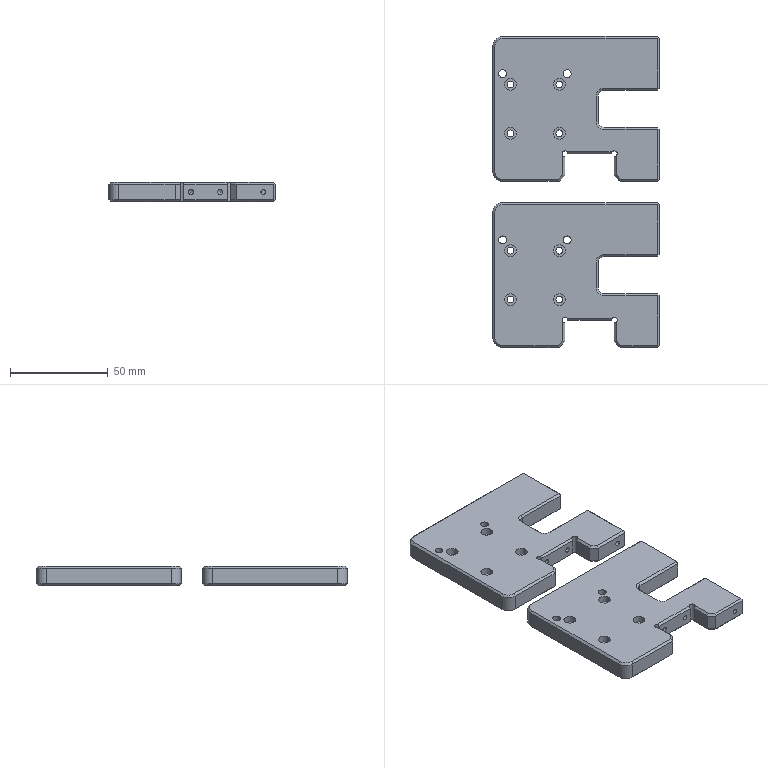NC program | NX | posted with a generic post | part box 85 x 159 x 10 mm
Whole program:
N10 G17 G21 G94 G90
(HOLE_MILLING_COPY_COPY_1 , TOOL : D4)
N12 T15 M6
N14 G54
N16 G17 G0 G90 X-30. Y0. B0. C0. S7500 M3
N18 G43 Z30. H15
N20 Z0.5
N22 G94 G3 X-30.45 Y0.45 R0.45 F1200.
N24 X-30.9 Y0. R0.45
N26 X-30.9 Y0. Z0.2 I0.9 J0.
N28 X-30.9 Y0. Z-0.1 I0.9 J0.
N30 X-30.9 Y0. Z-0.4 I0.9 J0.
N32 X-30.9 Y0. Z-0.7 I0.9 J0.
N34 X-30.9 Y0. Z-1. I0.9 J0.
N36 X-30.9 Y0. Z-1.3 I0.9 J0.
N38 X-30.9 Y0. Z-1.6 I0.9 J0.
N40 X-30.9 Y0. Z-1.9 I0.9 J0.
N42 X-30.9 Y0. Z-2.2 I0.9 J0.
N44 X-30.9 Y0. Z-2.5 I0.9 J0.
N46 X-30.9 Y0. Z-2.8 I0.9 J0.
N48 X-30.9 Y0. Z-3.1 I0.9 J0.
N50 X-30.9 Y0. Z-3.4 I0.9 J0.
N52 X-30.9 Y0. Z-3.7 I0.9 J0.
N54 X-30.9 Y0. Z-4. I0.9 J0.
N56 X-30.9 Y0. Z-4.3 I0.9 J0.
N58 X-30.9 Y0. Z-4.6 I0.9 J0.
N60 X-30.9 Y0. Z-4.9 I0.9 J0.
N62 X-30.9 Y0. Z-5.2 I0.9 J0.
N64 X-30.9 Y0. Z-5.5 I0.9 J0.
N66 X-30.9 Y0. Z-5.8 I0.9 J0.
N68 X-30.9 Y0. Z-6.1 I0.9 J0.
N70 X-30.9 Y0. Z-6.4 I0.9 J0.
N72 X-30.9 Y0. Z-6.7 I0.9 J0.
N74 X-30.9 Y0. Z-7. I0.9 J0.
N76 X-30.9 Y0. Z-7.3 I0.9 J0.
N78 X-30.9 Y0. Z-7.6 I0.9 J0.
N80 X-30.9 Y0. Z-7.9 I0.9 J0.
N82 X-30.9 Y0. Z-8.2 I0.9 J0.
N84 X-30.9 Y0. Z-8.5 I0.9 J0.
N86 X-30.9 Y0. Z-8.8 I0.9 J0.
N88 X-30.9 Y0. Z-9.1 I0.9 J0.
N90 X-30.9 Y0. Z-9.4 I0.9 J0.
N92 X-30.9 Y0. Z-9.7 I0.9 J0.
N94 X-30.9 Y0. Z-10. I0.9 J0.
N96 X-30.9 Y0. Z-10.3 I0.9 J0.
N98 X-30.9 Y0. Z-10.6 I0.9 J0.
N100 X-30.9 Y0. Z-10.9 I0.9 J0.
N102 X-30.9 Y0. Z-11.2 I0.9 J0.
N104 X-30.9 Y0. Z-11.5 I0.9 J0.
N106 X-30.9 Y0. Z-11.8 I0.9 J0.
N108 X-30.9 Y0. Z-12.1 I0.9 J0.
N110 X-30.9 Y0. Z-12.4 I0.9 J0.
N112 X-30.9 Y0. Z-12.7 I0.9 J0.
N114 X-30.9 Y0. Z-13. I0.9 J0.
N116 X-30.9 Y0. Z-13.3 I0.9 J0.
N118 X-30.9 Y0. Z-13.6 I0.9 J0.
N120 X-30.9 Y0. Z-13.9 I0.9 J0.
N122 X-30.9 Y0. Z-14.2 I0.9 J0.
N124 X-30.9 Y0. Z-14.5 I0.9 J0.
N126 X-30.9 Y0. Z-14.8 I0.9 J0.
N128 X-30.9 Y0. Z-15.1 I0.9 J0.
N130 X-30.9 Y0. Z-15.4 I0.9 J0.
N132 X-30.9 Y0. Z-15.7 I0.9 J0.
N134 X-30.9 Y0. Z-16. I0.9 J0.
N136 X-30. Y-0.9 R0.9
N138 X-30.9 Y0. R-0.9
N140 X-30.45 Y-0.45 R0.45
N142 X-30. Y0. R0.45
N144 G0 Z30.
N146 X30.
N148 Z0.5
N150 G3 X29.55 Y0.45 R0.45
N152 X29.1 Y0. R0.45
N154 X29.1 Y0. Z0.2 I0.9 J0.
N156 X29.1 Y0. Z-0.1 I0.9 J0.
N158 X29.1 Y0. Z-0.4 I0.9 J0.
N160 X29.1 Y0. Z-0.7 I0.9 J0.
N162 X29.1 Y0. Z-1. I0.9 J0.
N164 X29.1 Y0. Z-1.3 I0.9 J0.
N166 X29.1 Y0. Z-1.6 I0.9 J0.
N168 X29.1 Y0. Z-1.9 I0.9 J0.
N170 X29.1 Y0. Z-2.2 I0.9 J0.
N172 X29.1 Y0. Z-2.5 I0.9 J0.
N174 X29.1 Y0. Z-2.8 I0.9 J0.
N176 X29.1 Y0. Z-3.1 I0.9 J0.
N178 X29.1 Y0. Z-3.4 I0.9 J0.
N180 X29.1 Y0. Z-3.7 I0.9 J0.
N182 X29.1 Y0. Z-4. I0.9 J0.
N184 X29.1 Y0. Z-4.3 I0.9 J0.
N186 X29.1 Y0. Z-4.6 I0.9 J0.
N188 X29.1 Y0. Z-4.9 I0.9 J0.
N190 X29.1 Y0. Z-5.2 I0.9 J0.
N192 X29.1 Y0. Z-5.5 I0.9 J0.
N194 X29.1 Y0. Z-5.8 I0.9 J0.
N196 X29.1 Y0. Z-6.1 I0.9 J0.
N198 X29.1 Y0. Z-6.4 I0.9 J0.
N200 X29.1 Y0. Z-6.7 I0.9 J0.
N202 X29.1 Y0. Z-7. I0.9 J0.
N204 X29.1 Y0. Z-7.3 I0.9 J0.
N206 X29.1 Y0. Z-7.6 I0.9 J0.
N208 X29.1 Y0. Z-7.9 I0.9 J0.
N210 X29.1 Y0. Z-8.2 I0.9 J0.
N212 X29.1 Y0. Z-8.5 I0.9 J0.
N214 X29.1 Y0. Z-8.8 I0.9 J0.
N216 X29.1 Y0. Z-9.1 I0.9 J0.
N218 X29.1 Y0. Z-9.4 I0.9 J0.
N220 X29.1 Y0. Z-9.7 I0.9 J0.
N222 X29.1 Y0. Z-10. I0.9 J0.
N224 X29.1 Y0. Z-10.3 I0.9 J0.
N226 X29.1 Y0. Z-10.6 I0.9 J0.
N228 X29.1 Y0. Z-10.9 I0.9 J0.
N230 X29.1 Y0. Z-11.2 I0.9 J0.
N232 X29.1 Y0. Z-11.5 I0.9 J0.
N234 X29.1 Y0. Z-11.8 I0.9 J0.
N236 X29.1 Y0. Z-12.1 I0.9 J0.
N238 X29.1 Y0. Z-12.4 I0.9 J0.
N240 X29.1 Y0. Z-12.7 I0.9 J0.
N242 X29.1 Y0. Z-13. I0.9 J0.
N244 X29.1 Y0. Z-13.3 I0.9 J0.
N246 X29.1 Y0. Z-13.6 I0.9 J0.
N248 X29.1 Y0. Z-13.9 I0.9 J0.
N250 X29.1 Y0. Z-14.2 I0.9 J0.
N252 X29.1 Y0. Z-14.5 I0.9 J0.
N254 X29.1 Y0. Z-14.8 I0.9 J0.
N256 X29.1 Y0. Z-15.1 I0.9 J0.
N258 X29.1 Y0. Z-15.4 I0.9 J0.
N260 X29.1 Y0. Z-15.7 I0.9 J0.
N262 X29.1 Y0. Z-16. I0.9 J0.
N264 X30. Y-0.9 R0.9
N266 X29.1 Y0. R-0.9
N268 X29.55 Y-0.45 R0.45
N270 X30. Y0. R0.45
N272 G0 Z30.
N274 M5
(刀补13_COPY , TOOL : D4)
N276 M6
N278 G54
N280 G17 G0 G90 X-30. Y0. B0. C0. S7500 M3
N282 G43 Z30. H15
N284 Z0.5
N286 G41 G94 G1 X-30.004 Y0.1 F1000. D15
N288 G3 X-30.95 Y0. R0.478
N290 X-30.95 Y0. Z-0.5 I0.95 J0.
N292 X-30.95 Y0. Z-1.5 I0.95 J0.
N294 X-30.95 Y0. Z-2.5 I0.95 J0.
N296 X-30.95 Y0. Z-3.5 I0.95 J0.
N298 X-30.95 Y0. Z-4.5 I0.95 J0.
N300 X-30.95 Y0. Z-5.5 I0.95 J0.
N302 X-30.95 Y0. Z-6.5 I0.95 J0.
N304 X-30.95 Y0. Z-7.5 I0.95 J0.
N306 X-30.95 Y0. Z-8.5 I0.95 J0.
N308 X-30.95 Y0. Z-9.5 I0.95 J0.
N310 X-30.95 Y0. Z-10.5 I0.95 J0.
N312 X-30.95 Y0. Z-11.5 I0.95 J0.
N314 X-30.95 Y0. Z-12.5 I0.95 J0.
N316 X-30.95 Y0. Z-13.5 I0.95 J0.
N318 X-30.95 Y0. Z-14.5 I0.95 J0.
N320 X-30.95 Y0. Z-15.5 I0.95 J0.
N322 X-29.05 Y0. Z-16. I0.95 J0.
N324 X-30. Y0.95 R0.95
N326 X-29.05 Y0. R-0.95
N328 X-29.996 Y0.1 R0.478
N330 G40
N332 G1 X-30. Y0.
N334 G0 Z30.
N336 X30.
N338 Z0.5
N340 G41 G1 X29.996 Y0.1
N342 G3 X29.05 Y0. R0.478
N344 X29.05 Y0. Z-0.5 I0.95 J0.
N346 X29.05 Y0. Z-1.5 I0.95 J0.
N348 X29.05 Y0. Z-2.5 I0.95 J0.
N350 X29.05 Y0. Z-3.5 I0.95 J0.
N352 X29.05 Y0. Z-4.5 I0.95 J0.
N354 X29.05 Y0. Z-5.5 I0.95 J0.
N356 X29.05 Y0. Z-6.5 I0.95 J0.
N358 X29.05 Y0. Z-7.5 I0.95 J0.
N360 X29.05 Y0. Z-8.5 I0.95 J0.
N362 X29.05 Y0. Z-9.5 I0.95 J0.
N364 X29.05 Y0. Z-10.5 I0.95 J0.
N366 X29.05 Y0. Z-11.5 I0.95 J0.
N368 X29.05 Y0. Z-12.5 I0.95 J0.
N370 X29.05 Y0. Z-13.5 I0.95 J0.
N372 X29.05 Y0. Z-14.5 I0.95 J0.
N374 X29.05 Y0. Z-15.5 I0.95 J0.
N376 X30.95 Y0. Z-16. I0.95 J0.
N378 X30. Y0.95 R0.95
N380 X30.95 Y0. R-0.95
N382 X30.004 Y0.1 R0.478
N384 G40
N386 G1 X30. Y0.
N388 G0 Z30.
N390 M5
N392 M2